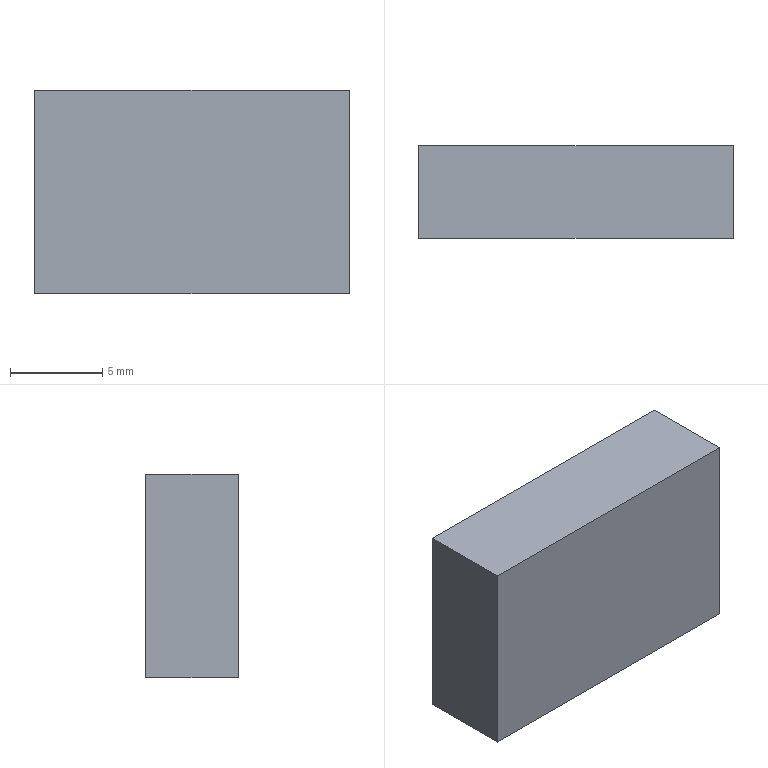Part | STEP file | PN_0019 Block_Default | 1 solid | 6 faces | box 17 x 5 x 11 mm | volume 935 mm3 | plane 6
STEP:
#1=CARTESIAN_POINT('',(0.,0.,0.));
#2=DIRECTION('',(0.,0.,1.));
#3=DIRECTION('',(1.,0.,0.));
#4=AXIS2_PLACEMENT_3D('',#1,#2,#3);
#5=CARTESIAN_POINT('',(-8.5,0.,-5.5));
#6=VERTEX_POINT('',#5);
#7=CARTESIAN_POINT('',(-8.5,0.,5.5));
#8=VERTEX_POINT('',#7);
#9=CARTESIAN_POINT('',(-8.5,0.,5.5));
#10=DIRECTION('',(0.,0.,1.));
#11=VECTOR('',#10,1.);
#12=LINE('',#9,#11);
#13=CARTESIAN_POINT('',(-8.5,5.,5.5));
#14=DIRECTION('',(1.,0.,0.));
#15=DIRECTION('',(0.,0.,-1.));
#16=AXIS2_PLACEMENT_3D('',#13,#14,#15);
#17=PLANE('',#16);
#18=CARTESIAN_POINT('',(0.,-5.));
#19=DIRECTION('',(-1.,0.));
#20=VECTOR('',#19,1.);
#21=LINE('',#18,#20);
#22=(GEOMETRIC_REPRESENTATION_CONTEXT(2)PARAMETRIC_REPRESENTATION_CONTEXT()REPRESENTATION_CONTEXT('',''));
#23=DEFINITIONAL_REPRESENTATION('',(#21),#22);
#24=PCURVE('',#17,#23);
#25=CARTESIAN_POINT('',(0.,0.,0.));
#26=DIRECTION('',(0.,1.,0.));
#27=DIRECTION('',(0.,0.,1.));
#28=AXIS2_PLACEMENT_3D('',#25,#26,#27);
#29=PLANE('',#28);
#30=CARTESIAN_POINT('',(5.5,-8.5));
#31=DIRECTION('',(1.,0.));
#32=VECTOR('',#31,1.);
#33=LINE('',#30,#32);
#34=(GEOMETRIC_REPRESENTATION_CONTEXT(2)PARAMETRIC_REPRESENTATION_CONTEXT()REPRESENTATION_CONTEXT('',''));
#35=DEFINITIONAL_REPRESENTATION('',(#33),#34);
#36=PCURVE('',#29,#35);
#37=SURFACE_CURVE('',#12,(#24,#36),.PCURVE_S1.);
#38=EDGE_CURVE('',#6,#8,#37,.T.);
#39=ORIENTED_EDGE('',*,*,#38,.T.);
#40=CARTESIAN_POINT('',(-8.5,5.,5.5));
#41=VERTEX_POINT('',#40);
#42=CARTESIAN_POINT('',(-8.5,5.,5.5));
#43=DIRECTION('',(0.,-1.,0.));
#44=VECTOR('',#43,1.);
#45=LINE('',#42,#44);
#46=CARTESIAN_POINT('',(0.,0.));
#47=DIRECTION('',(0.,-1.));
#48=VECTOR('',#47,1.);
#49=LINE('',#46,#48);
#50=(GEOMETRIC_REPRESENTATION_CONTEXT(2)PARAMETRIC_REPRESENTATION_CONTEXT()REPRESENTATION_CONTEXT('',''));
#51=DEFINITIONAL_REPRESENTATION('',(#49),#50);
#52=PCURVE('',#17,#51);
#53=CARTESIAN_POINT('',(8.5,5.,5.5));
#54=DIRECTION('',(0.,0.,-1.));
#55=DIRECTION('',(-1.,0.,0.));
#56=AXIS2_PLACEMENT_3D('',#53,#54,#55);
#57=PLANE('',#56);
#58=CARTESIAN_POINT('',(17.,0.));
#59=DIRECTION('',(0.,-1.));
#60=VECTOR('',#59,1.);
#61=LINE('',#58,#60);
#62=(GEOMETRIC_REPRESENTATION_CONTEXT(2)PARAMETRIC_REPRESENTATION_CONTEXT()REPRESENTATION_CONTEXT('',''));
#63=DEFINITIONAL_REPRESENTATION('',(#61),#62);
#64=PCURVE('',#57,#63);
#65=SURFACE_CURVE('',#45,(#52,#64),.PCURVE_S1.);
#66=EDGE_CURVE('',#41,#8,#65,.T.);
#67=ORIENTED_EDGE('',*,*,#66,.F.);
#68=CARTESIAN_POINT('',(-8.5,5.,-5.5));
#69=VERTEX_POINT('',#68);
#70=CARTESIAN_POINT('',(-8.5,5.,5.5));
#71=DIRECTION('',(0.,0.,1.));
#72=VECTOR('',#71,1.);
#73=LINE('',#70,#72);
#74=CARTESIAN_POINT('',(0.,0.));
#75=DIRECTION('',(-1.,0.));
#76=VECTOR('',#75,1.);
#77=LINE('',#74,#76);
#78=(GEOMETRIC_REPRESENTATION_CONTEXT(2)PARAMETRIC_REPRESENTATION_CONTEXT()REPRESENTATION_CONTEXT('',''));
#79=DEFINITIONAL_REPRESENTATION('',(#77),#78);
#80=PCURVE('',#17,#79);
#81=CARTESIAN_POINT('',(0.,5.,0.));
#82=DIRECTION('',(0.,1.,0.));
#83=DIRECTION('',(0.,0.,1.));
#84=AXIS2_PLACEMENT_3D('',#81,#82,#83);
#85=PLANE('',#84);
#86=CARTESIAN_POINT('',(5.5,-8.5));
#87=DIRECTION('',(1.,0.));
#88=VECTOR('',#87,1.);
#89=LINE('',#86,#88);
#90=(GEOMETRIC_REPRESENTATION_CONTEXT(2)PARAMETRIC_REPRESENTATION_CONTEXT()REPRESENTATION_CONTEXT('',''));
#91=DEFINITIONAL_REPRESENTATION('',(#89),#90);
#92=PCURVE('',#85,#91);
#93=SURFACE_CURVE('',#73,(#80,#92),.PCURVE_S1.);
#94=EDGE_CURVE('',#69,#41,#93,.T.);
#95=ORIENTED_EDGE('',*,*,#94,.F.);
#96=CARTESIAN_POINT('',(-8.5,5.,-5.5));
#97=DIRECTION('',(0.,-1.,0.));
#98=VECTOR('',#97,1.);
#99=LINE('',#96,#98);
#100=CARTESIAN_POINT('',(11.,0.));
#101=DIRECTION('',(0.,-1.));
#102=VECTOR('',#101,1.);
#103=LINE('',#100,#102);
#104=(GEOMETRIC_REPRESENTATION_CONTEXT(2)PARAMETRIC_REPRESENTATION_CONTEXT()REPRESENTATION_CONTEXT('',''));
#105=DEFINITIONAL_REPRESENTATION('',(#103),#104);
#106=PCURVE('',#17,#105);
#107=CARTESIAN_POINT('',(8.5,5.,-5.5));
#108=DIRECTION('',(0.,0.,1.));
#109=DIRECTION('',(1.,0.,0.));
#110=AXIS2_PLACEMENT_3D('',#107,#108,#109);
#111=PLANE('',#110);
#112=CARTESIAN_POINT('',(-17.,0.));
#113=DIRECTION('',(0.,-1.));
#114=VECTOR('',#113,1.);
#115=LINE('',#112,#114);
#116=(GEOMETRIC_REPRESENTATION_CONTEXT(2)PARAMETRIC_REPRESENTATION_CONTEXT()REPRESENTATION_CONTEXT('',''));
#117=DEFINITIONAL_REPRESENTATION('',(#115),#116);
#118=PCURVE('',#111,#117);
#119=SURFACE_CURVE('',#99,(#106,#118),.PCURVE_S1.);
#120=EDGE_CURVE('',#69,#6,#119,.T.);
#121=ORIENTED_EDGE('',*,*,#120,.T.);
#122=EDGE_LOOP('',(#39,#67,#95,#121));
#123=FACE_BOUND('',#122,.T.);
#124=ADVANCED_FACE('',(#123),#17,.F.);
#125=CARTESIAN_POINT('',(8.5,0.,5.5));
#126=VERTEX_POINT('',#125);
#127=CARTESIAN_POINT('',(8.5,0.,5.5));
#128=DIRECTION('',(1.,0.,0.));
#129=VECTOR('',#128,1.);
#130=LINE('',#127,#129);
#131=CARTESIAN_POINT('',(0.,-5.));
#132=DIRECTION('',(-1.,0.));
#133=VECTOR('',#132,1.);
#134=LINE('',#131,#133);
#135=(GEOMETRIC_REPRESENTATION_CONTEXT(2)PARAMETRIC_REPRESENTATION_CONTEXT()REPRESENTATION_CONTEXT('',''));
#136=DEFINITIONAL_REPRESENTATION('',(#134),#135);
#137=PCURVE('',#57,#136);
#138=CARTESIAN_POINT('',(5.5,8.5));
#139=DIRECTION('',(0.,1.));
#140=VECTOR('',#139,1.);
#141=LINE('',#138,#140);
#142=(GEOMETRIC_REPRESENTATION_CONTEXT(2)PARAMETRIC_REPRESENTATION_CONTEXT()REPRESENTATION_CONTEXT('',''));
#143=DEFINITIONAL_REPRESENTATION('',(#141),#142);
#144=PCURVE('',#29,#143);
#145=SURFACE_CURVE('',#130,(#137,#144),.PCURVE_S1.);
#146=EDGE_CURVE('',#8,#126,#145,.T.);
#147=ORIENTED_EDGE('',*,*,#146,.T.);
#148=CARTESIAN_POINT('',(8.5,5.,5.5));
#149=VERTEX_POINT('',#148);
#150=CARTESIAN_POINT('',(8.5,5.,5.5));
#151=DIRECTION('',(0.,-1.,0.));
#152=VECTOR('',#151,1.);
#153=LINE('',#150,#152);
#154=CARTESIAN_POINT('',(0.,0.));
#155=DIRECTION('',(0.,-1.));
#156=VECTOR('',#155,1.);
#157=LINE('',#154,#156);
#158=(GEOMETRIC_REPRESENTATION_CONTEXT(2)PARAMETRIC_REPRESENTATION_CONTEXT()REPRESENTATION_CONTEXT('',''));
#159=DEFINITIONAL_REPRESENTATION('',(#157),#158);
#160=PCURVE('',#57,#159);
#161=CARTESIAN_POINT('',(8.5,5.,5.5));
#162=DIRECTION('',(-1.,0.,0.));
#163=DIRECTION('',(0.,0.,1.));
#164=AXIS2_PLACEMENT_3D('',#161,#162,#163);
#165=PLANE('',#164);
#166=CARTESIAN_POINT('',(0.,0.));
#167=DIRECTION('',(0.,-1.));
#168=VECTOR('',#167,1.);
#169=LINE('',#166,#168);
#170=(GEOMETRIC_REPRESENTATION_CONTEXT(2)PARAMETRIC_REPRESENTATION_CONTEXT()REPRESENTATION_CONTEXT('',''));
#171=DEFINITIONAL_REPRESENTATION('',(#169),#170);
#172=PCURVE('',#165,#171);
#173=SURFACE_CURVE('',#153,(#160,#172),.PCURVE_S1.);
#174=EDGE_CURVE('',#149,#126,#173,.T.);
#175=ORIENTED_EDGE('',*,*,#174,.F.);
#176=CARTESIAN_POINT('',(8.5,5.,5.5));
#177=DIRECTION('',(1.,0.,0.));
#178=VECTOR('',#177,1.);
#179=LINE('',#176,#178);
#180=CARTESIAN_POINT('',(0.,0.));
#181=DIRECTION('',(-1.,0.));
#182=VECTOR('',#181,1.);
#183=LINE('',#180,#182);
#184=(GEOMETRIC_REPRESENTATION_CONTEXT(2)PARAMETRIC_REPRESENTATION_CONTEXT()REPRESENTATION_CONTEXT('',''));
#185=DEFINITIONAL_REPRESENTATION('',(#183),#184);
#186=PCURVE('',#57,#185);
#187=CARTESIAN_POINT('',(5.5,8.5));
#188=DIRECTION('',(0.,1.));
#189=VECTOR('',#188,1.);
#190=LINE('',#187,#189);
#191=(GEOMETRIC_REPRESENTATION_CONTEXT(2)PARAMETRIC_REPRESENTATION_CONTEXT()REPRESENTATION_CONTEXT('',''));
#192=DEFINITIONAL_REPRESENTATION('',(#190),#191);
#193=PCURVE('',#85,#192);
#194=SURFACE_CURVE('',#179,(#186,#193),.PCURVE_S1.);
#195=EDGE_CURVE('',#41,#149,#194,.T.);
#196=ORIENTED_EDGE('',*,*,#195,.F.);
#197=ORIENTED_EDGE('',*,*,#66,.T.);
#198=EDGE_LOOP('',(#147,#175,#196,#197));
#199=FACE_BOUND('',#198,.T.);
#200=ADVANCED_FACE('',(#199),#57,.F.);
#201=CARTESIAN_POINT('',(8.5,0.,-5.5));
#202=VERTEX_POINT('',#201);
#203=CARTESIAN_POINT('',(8.5,0.,5.5));
#204=DIRECTION('',(0.,0.,-1.));
#205=VECTOR('',#204,1.);
#206=LINE('',#203,#205);
#207=CARTESIAN_POINT('',(0.,-5.));
#208=DIRECTION('',(-1.,0.));
#209=VECTOR('',#208,1.);
#210=LINE('',#207,#209);
#211=(GEOMETRIC_REPRESENTATION_CONTEXT(2)PARAMETRIC_REPRESENTATION_CONTEXT()REPRESENTATION_CONTEXT('',''));
#212=DEFINITIONAL_REPRESENTATION('',(#210),#211);
#213=PCURVE('',#165,#212);
#214=CARTESIAN_POINT('',(5.5,8.5));
#215=DIRECTION('',(-1.,0.));
#216=VECTOR('',#215,1.);
#217=LINE('',#214,#216);
#218=(GEOMETRIC_REPRESENTATION_CONTEXT(2)PARAMETRIC_REPRESENTATION_CONTEXT()REPRESENTATION_CONTEXT('',''));
#219=DEFINITIONAL_REPRESENTATION('',(#217),#218);
#220=PCURVE('',#29,#219);
#221=SURFACE_CURVE('',#206,(#213,#220),.PCURVE_S1.);
#222=EDGE_CURVE('',#126,#202,#221,.T.);
#223=ORIENTED_EDGE('',*,*,#222,.T.);
#224=CARTESIAN_POINT('',(8.5,5.,-5.5));
#225=VERTEX_POINT('',#224);
#226=CARTESIAN_POINT('',(8.5,5.,-5.5));
#227=DIRECTION('',(0.,-1.,0.));
#228=VECTOR('',#227,1.);
#229=LINE('',#226,#228);
#230=CARTESIAN_POINT('',(-11.,0.));
#231=DIRECTION('',(0.,-1.));
#232=VECTOR('',#231,1.);
#233=LINE('',#230,#232);
#234=(GEOMETRIC_REPRESENTATION_CONTEXT(2)PARAMETRIC_REPRESENTATION_CONTEXT()REPRESENTATION_CONTEXT('',''));
#235=DEFINITIONAL_REPRESENTATION('',(#233),#234);
#236=PCURVE('',#165,#235);
#237=CARTESIAN_POINT('',(0.,0.));
#238=DIRECTION('',(0.,-1.));
#239=VECTOR('',#238,1.);
#240=LINE('',#237,#239);
#241=(GEOMETRIC_REPRESENTATION_CONTEXT(2)PARAMETRIC_REPRESENTATION_CONTEXT()REPRESENTATION_CONTEXT('',''));
#242=DEFINITIONAL_REPRESENTATION('',(#240),#241);
#243=PCURVE('',#111,#242);
#244=SURFACE_CURVE('',#229,(#236,#243),.PCURVE_S1.);
#245=EDGE_CURVE('',#225,#202,#244,.T.);
#246=ORIENTED_EDGE('',*,*,#245,.F.);
#247=CARTESIAN_POINT('',(8.5,5.,5.5));
#248=DIRECTION('',(0.,0.,-1.));
#249=VECTOR('',#248,1.);
#250=LINE('',#247,#249);
#251=CARTESIAN_POINT('',(0.,0.));
#252=DIRECTION('',(-1.,0.));
#253=VECTOR('',#252,1.);
#254=LINE('',#251,#253);
#255=(GEOMETRIC_REPRESENTATION_CONTEXT(2)PARAMETRIC_REPRESENTATION_CONTEXT()REPRESENTATION_CONTEXT('',''));
#256=DEFINITIONAL_REPRESENTATION('',(#254),#255);
#257=PCURVE('',#165,#256);
#258=CARTESIAN_POINT('',(5.5,8.5));
#259=DIRECTION('',(-1.,0.));
#260=VECTOR('',#259,1.);
#261=LINE('',#258,#260);
#262=(GEOMETRIC_REPRESENTATION_CONTEXT(2)PARAMETRIC_REPRESENTATION_CONTEXT()REPRESENTATION_CONTEXT('',''));
#263=DEFINITIONAL_REPRESENTATION('',(#261),#262);
#264=PCURVE('',#85,#263);
#265=SURFACE_CURVE('',#250,(#257,#264),.PCURVE_S1.);
#266=EDGE_CURVE('',#149,#225,#265,.T.);
#267=ORIENTED_EDGE('',*,*,#266,.F.);
#268=ORIENTED_EDGE('',*,*,#174,.T.);
#269=EDGE_LOOP('',(#223,#246,#267,#268));
#270=FACE_BOUND('',#269,.T.);
#271=ADVANCED_FACE('',(#270),#165,.F.);
#272=CARTESIAN_POINT('',(8.5,0.,-5.5));
#273=DIRECTION('',(-1.,0.,0.));
#274=VECTOR('',#273,1.);
#275=LINE('',#272,#274);
#276=CARTESIAN_POINT('',(0.,-5.));
#277=DIRECTION('',(-1.,0.));
#278=VECTOR('',#277,1.);
#279=LINE('',#276,#278);
#280=(GEOMETRIC_REPRESENTATION_CONTEXT(2)PARAMETRIC_REPRESENTATION_CONTEXT()REPRESENTATION_CONTEXT('',''));
#281=DEFINITIONAL_REPRESENTATION('',(#279),#280);
#282=PCURVE('',#111,#281);
#283=CARTESIAN_POINT('',(-5.5,8.5));
#284=DIRECTION('',(0.,-1.));
#285=VECTOR('',#284,1.);
#286=LINE('',#283,#285);
#287=(GEOMETRIC_REPRESENTATION_CONTEXT(2)PARAMETRIC_REPRESENTATION_CONTEXT()REPRESENTATION_CONTEXT('',''));
#288=DEFINITIONAL_REPRESENTATION('',(#286),#287);
#289=PCURVE('',#29,#288);
#290=SURFACE_CURVE('',#275,(#282,#289),.PCURVE_S1.);
#291=EDGE_CURVE('',#202,#6,#290,.T.);
#292=ORIENTED_EDGE('',*,*,#291,.T.);
#293=ORIENTED_EDGE('',*,*,#120,.F.);
#294=CARTESIAN_POINT('',(8.5,5.,-5.5));
#295=DIRECTION('',(-1.,0.,0.));
#296=VECTOR('',#295,1.);
#297=LINE('',#294,#296);
#298=CARTESIAN_POINT('',(0.,0.));
#299=DIRECTION('',(-1.,0.));
#300=VECTOR('',#299,1.);
#301=LINE('',#298,#300);
#302=(GEOMETRIC_REPRESENTATION_CONTEXT(2)PARAMETRIC_REPRESENTATION_CONTEXT()REPRESENTATION_CONTEXT('',''));
#303=DEFINITIONAL_REPRESENTATION('',(#301),#302);
#304=PCURVE('',#111,#303);
#305=CARTESIAN_POINT('',(-5.5,8.5));
#306=DIRECTION('',(0.,-1.));
#307=VECTOR('',#306,1.);
#308=LINE('',#305,#307);
#309=(GEOMETRIC_REPRESENTATION_CONTEXT(2)PARAMETRIC_REPRESENTATION_CONTEXT()REPRESENTATION_CONTEXT('',''));
#310=DEFINITIONAL_REPRESENTATION('',(#308),#309);
#311=PCURVE('',#85,#310);
#312=SURFACE_CURVE('',#297,(#304,#311),.PCURVE_S1.);
#313=EDGE_CURVE('',#225,#69,#312,.T.);
#314=ORIENTED_EDGE('',*,*,#313,.F.);
#315=ORIENTED_EDGE('',*,*,#245,.T.);
#316=EDGE_LOOP('',(#292,#293,#314,#315));
#317=FACE_BOUND('',#316,.T.);
#318=ADVANCED_FACE('',(#317),#111,.F.);
#319=ORIENTED_EDGE('',*,*,#94,.T.);
#320=ORIENTED_EDGE('',*,*,#195,.T.);
#321=ORIENTED_EDGE('',*,*,#266,.T.);
#322=ORIENTED_EDGE('',*,*,#313,.T.);
#323=EDGE_LOOP('',(#319,#320,#321,#322));
#324=FACE_BOUND('',#323,.T.);
#325=ADVANCED_FACE('',(#324),#85,.T.);
#326=ORIENTED_EDGE('',*,*,#38,.F.);
#327=ORIENTED_EDGE('',*,*,#291,.F.);
#328=ORIENTED_EDGE('',*,*,#222,.F.);
#329=ORIENTED_EDGE('',*,*,#146,.F.);
#330=EDGE_LOOP('',(#326,#327,#328,#329));
#331=FACE_BOUND('',#330,.T.);
#332=ADVANCED_FACE('',(#331),#29,.F.);
#333=CLOSED_SHELL('',(#124,#200,#271,#318,#325,#332));
#334=MANIFOLD_SOLID_BREP('',#333);
#335=(LENGTH_UNIT()NAMED_UNIT(*)SI_UNIT(.MILLI.,.METRE.));
#336=UNCERTAINTY_MEASURE_WITH_UNIT(LENGTH_MEASURE(0.0000001),#335,'','');
#337=(NAMED_UNIT(*)PLANE_ANGLE_UNIT()SI_UNIT($,.RADIAN.));
#338=(NAMED_UNIT(*)SI_UNIT($,.STERADIAN.)SOLID_ANGLE_UNIT());
#339=(GEOMETRIC_REPRESENTATION_CONTEXT(3)GLOBAL_UNCERTAINTY_ASSIGNED_CONTEXT((#336))GLOBAL_UNIT_ASSIGNED_CONTEXT((#335,#337,#338))REPRESENTATION_CONTEXT('',''));
#340=ADVANCED_BREP_SHAPE_REPRESENTATION('',(#4,#334),#339);